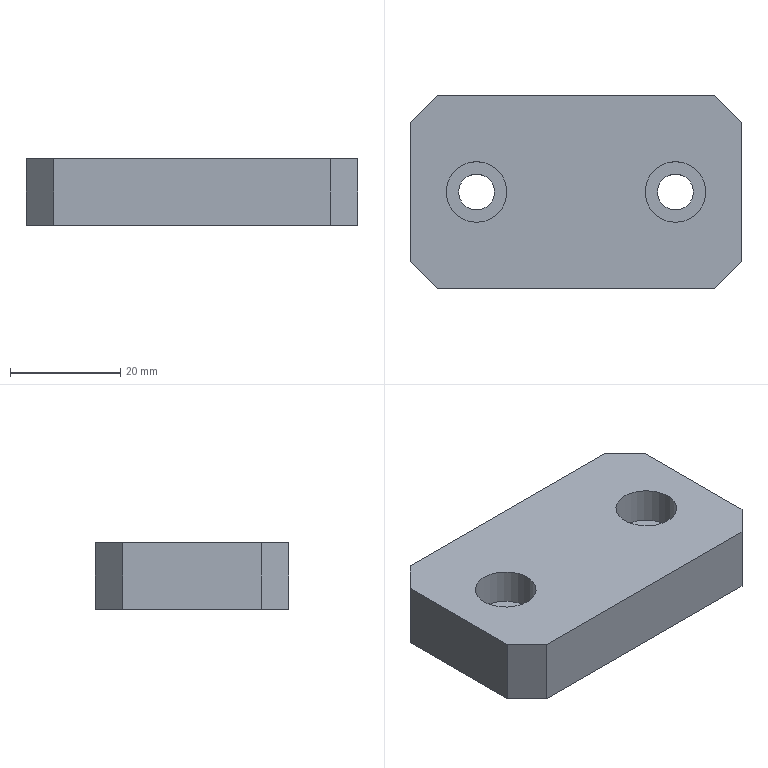Part | STEP file | lll_id370_x_t | 1 solid | 125 faces | box 60 x 35 x 12 mm | volume 22990 mm3 | other 64 | plane 57 | cylinder 4 | commonest cylinder face diameters 6.5 x2 11 x2